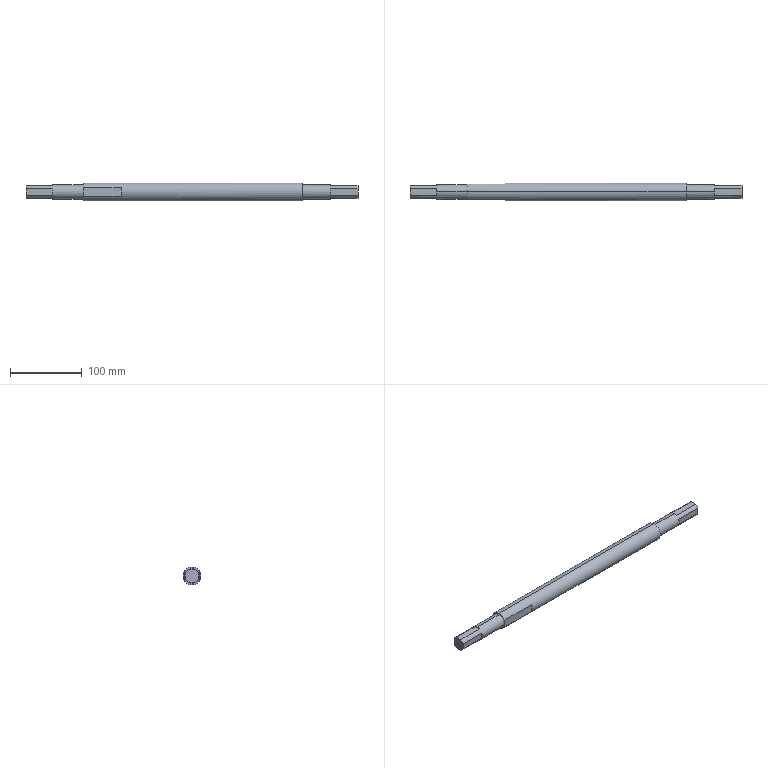Part | STEP file | shaft 3_SUS304 | 1 solid | 30 faces | box 463.7 x 25 x 25 mm | volume 196661 mm3 | plane 24 | cylinder 6 | commonest cylinder face diameters 20 x4 25 x2